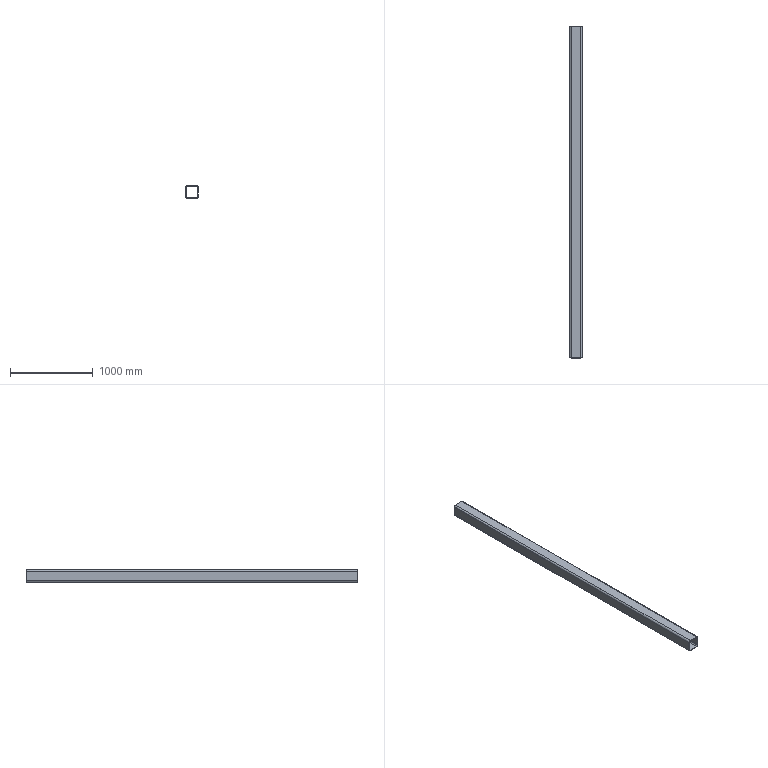Part | SolidWorks | features ICE 2, Extrusion 1, LPattern 1 | 1 solid | 298 faces | box 150 x 4000 x 150 mm | volume 16889916 mm3 | cylinder 276 | plane 22 | commonest cylinder face diameters 5.2 x268 24 x4 40 x4